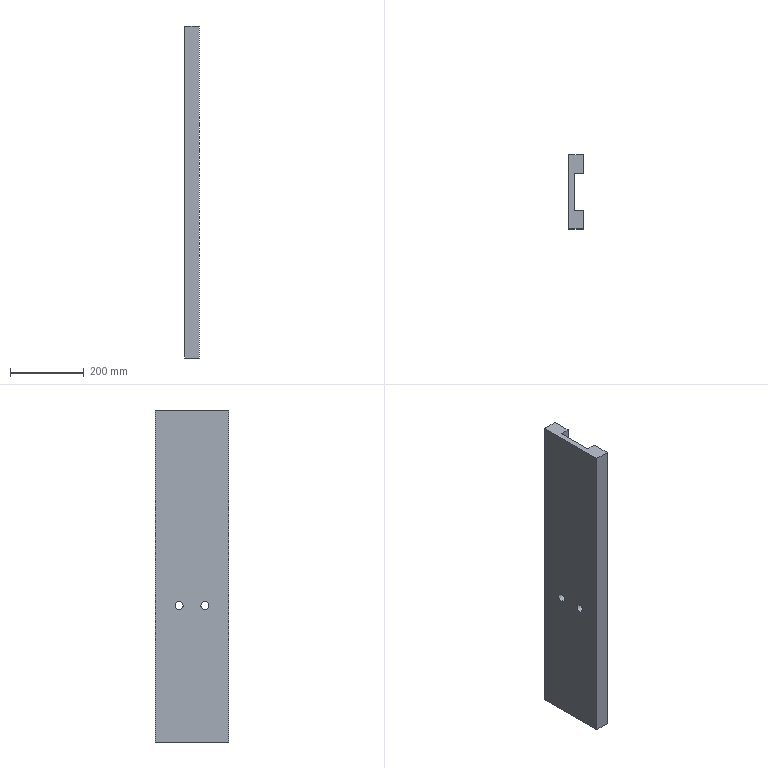Part | SolidWorks | features 3DProfileFeature 1, Extrusion 1, HoleWzd 1 | 1 solid | 14 faces | box 40 x 200 x 900 mm | volume 4927112 mm3 | plane 10 | cylinder 4 | commonest cylinder face diameters 22.225 x4
STEP:
#1=CARTESIAN_POINT('',(0.,135.,381.112));
#2=VERTEX_POINT('',#1);
#3=CARTESIAN_POINT('',(0.,135.,358.888));
#4=VERTEX_POINT('',#3);
#5=CARTESIAN_POINT('',(0.,135.,370.));
#6=DIRECTION('',(1.,0.,0.));
#7=DIRECTION('',(0.,0.,-1.));
#8=AXIS2_PLACEMENT_3D('',#5,#6,#7);
#9=CIRCLE('',#8,11.112);
#10=EDGE_CURVE('',#2,#4,#9,.T.);
#11=ORIENTED_EDGE('',*,*,#10,.F.);
#12=CARTESIAN_POINT('',(15.,135.,381.112));
#13=VERTEX_POINT('',#12);
#14=CARTESIAN_POINT('',(15.,135.,381.112));
#15=DIRECTION('',(1.,0.,0.));
#16=VECTOR('',#15,1000.);
#17=LINE('',#14,#16);
#18=EDGE_CURVE('',#2,#13,#17,.T.);
#19=ORIENTED_EDGE('',*,*,#18,.T.);
#20=CARTESIAN_POINT('',(15.,135.,358.888));
#21=VERTEX_POINT('',#20);
#22=CARTESIAN_POINT('',(15.,135.,370.));
#23=DIRECTION('',(1.,0.,0.));
#24=DIRECTION('',(0.,0.,-1.));
#25=AXIS2_PLACEMENT_3D('',#22,#23,#24);
#26=CIRCLE('',#25,11.112);
#27=EDGE_CURVE('',#13,#21,#26,.T.);
#28=ORIENTED_EDGE('',*,*,#27,.T.);
#29=CARTESIAN_POINT('',(15.,135.,358.888));
#30=DIRECTION('',(1.,0.,0.));
#31=VECTOR('',#30,1000.);
#32=LINE('',#29,#31);
#33=EDGE_CURVE('',#4,#21,#32,.T.);
#34=ORIENTED_EDGE('',*,*,#33,.F.);
#35=EDGE_LOOP('',(#11,#19,#28,#34));
#36=FACE_OUTER_BOUND('',#35,.T.);
#37=CARTESIAN_POINT('',(15.,135.,370.));
#38=DIRECTION('',(1.,0.,0.));
#39=DIRECTION('',(0.,0.,-1.));
#40=AXIS2_PLACEMENT_3D('',#37,#38,#39);
#41=CYLINDRICAL_SURFACE('',#40,11.112);
#42=ADVANCED_FACE('',(#36),#41,.F.);
#43=CARTESIAN_POINT('',(0.,65.,381.112));
#44=VERTEX_POINT('',#43);
#45=CARTESIAN_POINT('',(0.,65.,358.888));
#46=VERTEX_POINT('',#45);
#47=CARTESIAN_POINT('',(0.,65.,370.));
#48=DIRECTION('',(1.,0.,0.));
#49=DIRECTION('',(0.,0.,-1.));
#50=AXIS2_PLACEMENT_3D('',#47,#48,#49);
#51=CIRCLE('',#50,11.112);
#52=EDGE_CURVE('',#44,#46,#51,.T.);
#53=ORIENTED_EDGE('',*,*,#52,.F.);
#54=CARTESIAN_POINT('',(15.,65.,381.112));
#55=VERTEX_POINT('',#54);
#56=CARTESIAN_POINT('',(15.,65.,381.112));
#57=DIRECTION('',(1.,0.,0.));
#58=VECTOR('',#57,1000.);
#59=LINE('',#56,#58);
#60=EDGE_CURVE('',#44,#55,#59,.T.);
#61=ORIENTED_EDGE('',*,*,#60,.T.);
#62=CARTESIAN_POINT('',(15.,65.,358.888));
#63=VERTEX_POINT('',#62);
#64=CARTESIAN_POINT('',(15.,65.,370.));
#65=DIRECTION('',(1.,0.,0.));
#66=DIRECTION('',(0.,0.,-1.));
#67=AXIS2_PLACEMENT_3D('',#64,#65,#66);
#68=CIRCLE('',#67,11.112);
#69=EDGE_CURVE('',#55,#63,#68,.T.);
#70=ORIENTED_EDGE('',*,*,#69,.T.);
#71=CARTESIAN_POINT('',(15.,65.,358.888));
#72=DIRECTION('',(1.,0.,0.));
#73=VECTOR('',#72,1000.);
#74=LINE('',#71,#73);
#75=EDGE_CURVE('',#46,#63,#74,.T.);
#76=ORIENTED_EDGE('',*,*,#75,.F.);
#77=EDGE_LOOP('',(#53,#61,#70,#76));
#78=FACE_OUTER_BOUND('',#77,.T.);
#79=CARTESIAN_POINT('',(15.,65.,370.));
#80=DIRECTION('',(1.,0.,0.));
#81=DIRECTION('',(0.,0.,-1.));
#82=AXIS2_PLACEMENT_3D('',#79,#80,#81);
#83=CYLINDRICAL_SURFACE('',#82,11.112);
#84=ADVANCED_FACE('',(#78),#83,.F.);
#85=CARTESIAN_POINT('',(0.,0.,0.));
#86=VERTEX_POINT('',#85);
#87=CARTESIAN_POINT('',(40.,0.,0.));
#88=VERTEX_POINT('',#87);
#89=CARTESIAN_POINT('',(40.,0.,0.));
#90=DIRECTION('',(1.,0.,0.));
#91=VECTOR('',#90,1000.);
#92=LINE('',#89,#91);
#93=EDGE_CURVE('',#86,#88,#92,.T.);
#94=ORIENTED_EDGE('',*,*,#93,.T.);
#95=CARTESIAN_POINT('',(40.,0.,900.));
#96=VERTEX_POINT('',#95);
#97=CARTESIAN_POINT('',(40.,0.,900.));
#98=DIRECTION('',(0.,0.,-1.));
#99=VECTOR('',#98,1000.);
#100=LINE('',#97,#99);
#101=EDGE_CURVE('',#96,#88,#100,.T.);
#102=ORIENTED_EDGE('',*,*,#101,.F.);
#103=CARTESIAN_POINT('',(0.,0.,900.));
#104=VERTEX_POINT('',#103);
#105=CARTESIAN_POINT('',(40.,0.,900.));
#106=DIRECTION('',(1.,0.,0.));
#107=VECTOR('',#106,1000.);
#108=LINE('',#105,#107);
#109=EDGE_CURVE('',#104,#96,#108,.T.);
#110=ORIENTED_EDGE('',*,*,#109,.F.);
#111=CARTESIAN_POINT('',(0.,0.,900.));
#112=DIRECTION('',(0.,0.,-1.));
#113=VECTOR('',#112,1000.);
#114=LINE('',#111,#113);
#115=EDGE_CURVE('',#104,#86,#114,.T.);
#116=ORIENTED_EDGE('',*,*,#115,.T.);
#117=EDGE_LOOP('',(#94,#102,#110,#116));
#118=FACE_OUTER_BOUND('',#117,.T.);
#119=CARTESIAN_POINT('',(40.,0.,900.));
#120=DIRECTION('',(0.,1.,0.));
#121=DIRECTION('',(-1.,0.,0.));
#122=AXIS2_PLACEMENT_3D('',#119,#120,#121);
#123=PLANE('',#122);
#124=ADVANCED_FACE('',(#118),#123,.F.);
#125=CARTESIAN_POINT('',(40.,49.75,0.));
#126=VERTEX_POINT('',#125);
#127=CARTESIAN_POINT('',(40.,49.75,0.));
#128=DIRECTION('',(0.,1.,0.));
#129=VECTOR('',#128,1000.);
#130=LINE('',#127,#129);
#131=EDGE_CURVE('',#88,#126,#130,.T.);
#132=ORIENTED_EDGE('',*,*,#131,.T.);
#133=CARTESIAN_POINT('',(40.,49.75,900.));
#134=VERTEX_POINT('',#133);
#135=CARTESIAN_POINT('',(40.,49.75,900.));
#136=DIRECTION('',(0.,0.,-1.));
#137=VECTOR('',#136,1000.);
#138=LINE('',#135,#137);
#139=EDGE_CURVE('',#134,#126,#138,.T.);
#140=ORIENTED_EDGE('',*,*,#139,.F.);
#141=CARTESIAN_POINT('',(40.,49.75,900.));
#142=DIRECTION('',(0.,1.,0.));
#143=VECTOR('',#142,1000.);
#144=LINE('',#141,#143);
#145=EDGE_CURVE('',#96,#134,#144,.T.);
#146=ORIENTED_EDGE('',*,*,#145,.F.);
#147=ORIENTED_EDGE('',*,*,#101,.T.);
#148=EDGE_LOOP('',(#132,#140,#146,#147));
#149=FACE_OUTER_BOUND('',#148,.T.);
#150=CARTESIAN_POINT('',(40.,49.75,900.));
#151=DIRECTION('',(-1.,0.,0.));
#152=DIRECTION('',(0.,-1.,0.));
#153=AXIS2_PLACEMENT_3D('',#150,#151,#152);
#154=PLANE('',#153);
#155=ADVANCED_FACE('',(#149),#154,.F.);
#156=CARTESIAN_POINT('',(15.,49.75,0.));
#157=VERTEX_POINT('',#156);
#158=CARTESIAN_POINT('',(15.,49.75,0.));
#159=DIRECTION('',(-1.,0.,0.));
#160=VECTOR('',#159,1000.);
#161=LINE('',#158,#160);
#162=EDGE_CURVE('',#126,#157,#161,.T.);
#163=ORIENTED_EDGE('',*,*,#162,.T.);
#164=CARTESIAN_POINT('',(15.,49.75,900.));
#165=VERTEX_POINT('',#164);
#166=CARTESIAN_POINT('',(15.,49.75,900.));
#167=DIRECTION('',(0.,0.,-1.));
#168=VECTOR('',#167,1000.);
#169=LINE('',#166,#168);
#170=EDGE_CURVE('',#165,#157,#169,.T.);
#171=ORIENTED_EDGE('',*,*,#170,.F.);
#172=CARTESIAN_POINT('',(15.,49.75,900.));
#173=DIRECTION('',(-1.,0.,0.));
#174=VECTOR('',#173,1000.);
#175=LINE('',#172,#174);
#176=EDGE_CURVE('',#134,#165,#175,.T.);
#177=ORIENTED_EDGE('',*,*,#176,.F.);
#178=ORIENTED_EDGE('',*,*,#139,.T.);
#179=EDGE_LOOP('',(#163,#171,#177,#178));
#180=FACE_OUTER_BOUND('',#179,.T.);
#181=CARTESIAN_POINT('',(15.,49.75,900.));
#182=DIRECTION('',(0.,-1.,0.));
#183=DIRECTION('',(0.,0.,-1.));
#184=AXIS2_PLACEMENT_3D('',#181,#182,#183);
#185=PLANE('',#184);
#186=ADVANCED_FACE('',(#180),#185,.F.);
#187=CARTESIAN_POINT('',(15.,135.,370.));
#188=DIRECTION('',(1.,0.,0.));
#189=DIRECTION('',(0.,0.,-1.));
#190=AXIS2_PLACEMENT_3D('',#187,#188,#189);
#191=CIRCLE('',#190,11.112);
#192=EDGE_CURVE('',#21,#13,#191,.T.);
#193=ORIENTED_EDGE('',*,*,#192,.F.);
#194=ORIENTED_EDGE('',*,*,#27,.F.);
#195=EDGE_LOOP('',(#193,#194));
#196=FACE_BOUND('',#195,.T.);
#197=CARTESIAN_POINT('',(15.,65.,370.));
#198=DIRECTION('',(1.,0.,0.));
#199=DIRECTION('',(0.,0.,-1.));
#200=AXIS2_PLACEMENT_3D('',#197,#198,#199);
#201=CIRCLE('',#200,11.112);
#202=EDGE_CURVE('',#63,#55,#201,.T.);
#203=ORIENTED_EDGE('',*,*,#202,.F.);
#204=ORIENTED_EDGE('',*,*,#69,.F.);
#205=EDGE_LOOP('',(#203,#204));
#206=FACE_BOUND('',#205,.T.);
#207=CARTESIAN_POINT('',(15.,150.25,0.));
#208=VERTEX_POINT('',#207);
#209=CARTESIAN_POINT('',(15.,150.25,0.));
#210=DIRECTION('',(0.,1.,0.));
#211=VECTOR('',#210,1000.);
#212=LINE('',#209,#211);
#213=EDGE_CURVE('',#157,#208,#212,.T.);
#214=ORIENTED_EDGE('',*,*,#213,.T.);
#215=CARTESIAN_POINT('',(15.,150.25,900.));
#216=VERTEX_POINT('',#215);
#217=CARTESIAN_POINT('',(15.,150.25,900.));
#218=DIRECTION('',(0.,0.,-1.));
#219=VECTOR('',#218,1000.);
#220=LINE('',#217,#219);
#221=EDGE_CURVE('',#216,#208,#220,.T.);
#222=ORIENTED_EDGE('',*,*,#221,.F.);
#223=CARTESIAN_POINT('',(15.,150.25,900.));
#224=DIRECTION('',(0.,1.,0.));
#225=VECTOR('',#224,1000.);
#226=LINE('',#223,#225);
#227=EDGE_CURVE('',#165,#216,#226,.T.);
#228=ORIENTED_EDGE('',*,*,#227,.F.);
#229=ORIENTED_EDGE('',*,*,#170,.T.);
#230=EDGE_LOOP('',(#214,#222,#228,#229));
#231=FACE_OUTER_BOUND('',#230,.T.);
#232=CARTESIAN_POINT('',(15.,150.25,900.));
#233=DIRECTION('',(-1.,0.,0.));
#234=DIRECTION('',(0.,-1.,0.));
#235=AXIS2_PLACEMENT_3D('',#232,#233,#234);
#236=PLANE('',#235);
#237=ADVANCED_FACE('',(#196,#206,#231),#236,.F.);
#238=CARTESIAN_POINT('',(40.,150.25,0.));
#239=VERTEX_POINT('',#238);
#240=CARTESIAN_POINT('',(40.,150.25,0.));
#241=DIRECTION('',(1.,0.,0.));
#242=VECTOR('',#241,1000.);
#243=LINE('',#240,#242);
#244=EDGE_CURVE('',#208,#239,#243,.T.);
#245=ORIENTED_EDGE('',*,*,#244,.T.);
#246=CARTESIAN_POINT('',(40.,150.25,900.));
#247=VERTEX_POINT('',#246);
#248=CARTESIAN_POINT('',(40.,150.25,900.));
#249=DIRECTION('',(0.,0.,-1.));
#250=VECTOR('',#249,1000.);
#251=LINE('',#248,#250);
#252=EDGE_CURVE('',#247,#239,#251,.T.);
#253=ORIENTED_EDGE('',*,*,#252,.F.);
#254=CARTESIAN_POINT('',(40.,150.25,900.));
#255=DIRECTION('',(1.,0.,0.));
#256=VECTOR('',#255,1000.);
#257=LINE('',#254,#256);
#258=EDGE_CURVE('',#216,#247,#257,.T.);
#259=ORIENTED_EDGE('',*,*,#258,.F.);
#260=ORIENTED_EDGE('',*,*,#221,.T.);
#261=EDGE_LOOP('',(#245,#253,#259,#260));
#262=FACE_OUTER_BOUND('',#261,.T.);
#263=CARTESIAN_POINT('',(40.,150.25,900.));
#264=DIRECTION('',(0.,1.,0.));
#265=DIRECTION('',(0.,0.,1.));
#266=AXIS2_PLACEMENT_3D('',#263,#264,#265);
#267=PLANE('',#266);
#268=ADVANCED_FACE('',(#262),#267,.F.);
#269=CARTESIAN_POINT('',(40.,200.,0.));
#270=VERTEX_POINT('',#269);
#271=CARTESIAN_POINT('',(40.,200.,0.));
#272=DIRECTION('',(0.,1.,0.));
#273=VECTOR('',#272,1000.);
#274=LINE('',#271,#273);
#275=EDGE_CURVE('',#239,#270,#274,.T.);
#276=ORIENTED_EDGE('',*,*,#275,.T.);
#277=CARTESIAN_POINT('',(40.,200.,900.));
#278=VERTEX_POINT('',#277);
#279=CARTESIAN_POINT('',(40.,200.,900.));
#280=DIRECTION('',(0.,0.,-1.));
#281=VECTOR('',#280,1000.);
#282=LINE('',#279,#281);
#283=EDGE_CURVE('',#278,#270,#282,.T.);
#284=ORIENTED_EDGE('',*,*,#283,.F.);
#285=CARTESIAN_POINT('',(40.,200.,900.));
#286=DIRECTION('',(0.,1.,0.));
#287=VECTOR('',#286,1000.);
#288=LINE('',#285,#287);
#289=EDGE_CURVE('',#247,#278,#288,.T.);
#290=ORIENTED_EDGE('',*,*,#289,.F.);
#291=ORIENTED_EDGE('',*,*,#252,.T.);
#292=EDGE_LOOP('',(#276,#284,#290,#291));
#293=FACE_OUTER_BOUND('',#292,.T.);
#294=CARTESIAN_POINT('',(40.,200.,900.));
#295=DIRECTION('',(-1.,0.,0.));
#296=DIRECTION('',(0.,-1.,0.));
#297=AXIS2_PLACEMENT_3D('',#294,#295,#296);
#298=PLANE('',#297);
#299=ADVANCED_FACE('',(#293),#298,.F.);
#300=CARTESIAN_POINT('',(0.,200.,0.));
#301=VERTEX_POINT('',#300);
#302=CARTESIAN_POINT('',(0.,200.,0.));
#303=DIRECTION('',(-1.,0.,0.));
#304=VECTOR('',#303,1000.);
#305=LINE('',#302,#304);
#306=EDGE_CURVE('',#270,#301,#305,.T.);
#307=ORIENTED_EDGE('',*,*,#306,.T.);
#308=CARTESIAN_POINT('',(0.,200.,900.));
#309=VERTEX_POINT('',#308);
#310=CARTESIAN_POINT('',(0.,200.,900.));
#311=DIRECTION('',(0.,0.,-1.));
#312=VECTOR('',#311,1000.);
#313=LINE('',#310,#312);
#314=EDGE_CURVE('',#309,#301,#313,.T.);
#315=ORIENTED_EDGE('',*,*,#314,.F.);
#316=CARTESIAN_POINT('',(0.,200.,900.));
#317=DIRECTION('',(-1.,0.,0.));
#318=VECTOR('',#317,1000.);
#319=LINE('',#316,#318);
#320=EDGE_CURVE('',#278,#309,#319,.T.);
#321=ORIENTED_EDGE('',*,*,#320,.F.);
#322=ORIENTED_EDGE('',*,*,#283,.T.);
#323=EDGE_LOOP('',(#307,#315,#321,#322));
#324=FACE_OUTER_BOUND('',#323,.T.);
#325=CARTESIAN_POINT('',(0.,200.,900.));
#326=DIRECTION('',(0.,-1.,0.));
#327=DIRECTION('',(0.,0.,-1.));
#328=AXIS2_PLACEMENT_3D('',#325,#326,#327);
#329=PLANE('',#328);
#330=ADVANCED_FACE('',(#324),#329,.F.);
#331=CARTESIAN_POINT('',(0.,135.,370.));
#332=DIRECTION('',(1.,0.,0.));
#333=DIRECTION('',(0.,0.,-1.));
#334=AXIS2_PLACEMENT_3D('',#331,#332,#333);
#335=CIRCLE('',#334,11.112);
#336=EDGE_CURVE('',#4,#2,#335,.T.);
#337=ORIENTED_EDGE('',*,*,#336,.T.);
#338=ORIENTED_EDGE('',*,*,#10,.T.);
#339=EDGE_LOOP('',(#337,#338));
#340=FACE_BOUND('',#339,.T.);
#341=CARTESIAN_POINT('',(0.,65.,370.));
#342=DIRECTION('',(1.,0.,0.));
#343=DIRECTION('',(0.,0.,-1.));
#344=AXIS2_PLACEMENT_3D('',#341,#342,#343);
#345=CIRCLE('',#344,11.112);
#346=EDGE_CURVE('',#46,#44,#345,.T.);
#347=ORIENTED_EDGE('',*,*,#346,.T.);
#348=ORIENTED_EDGE('',*,*,#52,.T.);
#349=EDGE_LOOP('',(#347,#348));
#350=FACE_BOUND('',#349,.T.);
#351=CARTESIAN_POINT('',(0.,0.,0.));
#352=DIRECTION('',(0.,-1.,0.));
#353=VECTOR('',#352,1000.);
#354=LINE('',#351,#353);
#355=EDGE_CURVE('',#301,#86,#354,.T.);
#356=ORIENTED_EDGE('',*,*,#355,.T.);
#357=ORIENTED_EDGE('',*,*,#115,.F.);
#358=CARTESIAN_POINT('',(0.,0.,900.));
#359=DIRECTION('',(0.,-1.,0.));
#360=VECTOR('',#359,1000.);
#361=LINE('',#358,#360);
#362=EDGE_CURVE('',#309,#104,#361,.T.);
#363=ORIENTED_EDGE('',*,*,#362,.F.);
#364=ORIENTED_EDGE('',*,*,#314,.T.);
#365=EDGE_LOOP('',(#356,#357,#363,#364));
#366=FACE_OUTER_BOUND('',#365,.T.);
#367=CARTESIAN_POINT('',(0.,0.,900.));
#368=DIRECTION('',(1.,0.,0.));
#369=DIRECTION('',(0.,0.,-1.));
#370=AXIS2_PLACEMENT_3D('',#367,#368,#369);
#371=PLANE('',#370);
#372=ADVANCED_FACE('',(#340,#350,#366),#371,.F.);
#373=ORIENTED_EDGE('',*,*,#109,.T.);
#374=ORIENTED_EDGE('',*,*,#145,.T.);
#375=ORIENTED_EDGE('',*,*,#176,.T.);
#376=ORIENTED_EDGE('',*,*,#227,.T.);
#377=ORIENTED_EDGE('',*,*,#258,.T.);
#378=ORIENTED_EDGE('',*,*,#289,.T.);
#379=ORIENTED_EDGE('',*,*,#320,.T.);
#380=ORIENTED_EDGE('',*,*,#362,.T.);
#381=EDGE_LOOP('',(#373,#374,#375,#376,#377,#378,#379,#380));
#382=FACE_OUTER_BOUND('',#381,.T.);
#383=CARTESIAN_POINT('',(0.,0.,900.));
#384=DIRECTION('',(0.,0.,-1.));
#385=DIRECTION('',(-1.,0.,0.));
#386=AXIS2_PLACEMENT_3D('',#383,#384,#385);
#387=PLANE('',#386);
#388=ADVANCED_FACE('',(#382),#387,.F.);
#389=ORIENTED_EDGE('',*,*,#93,.F.);
#390=ORIENTED_EDGE('',*,*,#355,.F.);
#391=ORIENTED_EDGE('',*,*,#306,.F.);
#392=ORIENTED_EDGE('',*,*,#275,.F.);
#393=ORIENTED_EDGE('',*,*,#244,.F.);
#394=ORIENTED_EDGE('',*,*,#213,.F.);
#395=ORIENTED_EDGE('',*,*,#162,.F.);
#396=ORIENTED_EDGE('',*,*,#131,.F.);
#397=EDGE_LOOP('',(#389,#390,#391,#392,#393,#394,#395,#396));
#398=FACE_OUTER_BOUND('',#397,.T.);
#399=CARTESIAN_POINT('',(0.,0.,0.));
#400=DIRECTION('',(0.,0.,-1.));
#401=DIRECTION('',(-1.,0.,0.));
#402=AXIS2_PLACEMENT_3D('',#399,#400,#401);
#403=PLANE('',#402);
#404=ADVANCED_FACE('',(#398),#403,.T.);
#405=ORIENTED_EDGE('',*,*,#60,.F.);
#406=ORIENTED_EDGE('',*,*,#346,.F.);
#407=ORIENTED_EDGE('',*,*,#75,.T.);
#408=ORIENTED_EDGE('',*,*,#202,.T.);
#409=EDGE_LOOP('',(#405,#406,#407,#408));
#410=FACE_OUTER_BOUND('',#409,.T.);
#411=CARTESIAN_POINT('',(15.,65.,370.));
#412=DIRECTION('',(1.,0.,0.));
#413=DIRECTION('',(0.,0.,-1.));
#414=AXIS2_PLACEMENT_3D('',#411,#412,#413);
#415=CYLINDRICAL_SURFACE('',#414,11.112);
#416=ADVANCED_FACE('',(#410),#415,.F.);
#417=ORIENTED_EDGE('',*,*,#18,.F.);
#418=ORIENTED_EDGE('',*,*,#336,.F.);
#419=ORIENTED_EDGE('',*,*,#33,.T.);
#420=ORIENTED_EDGE('',*,*,#192,.T.);
#421=EDGE_LOOP('',(#417,#418,#419,#420));
#422=FACE_OUTER_BOUND('',#421,.T.);
#423=CARTESIAN_POINT('',(15.,135.,370.));
#424=DIRECTION('',(1.,0.,0.));
#425=DIRECTION('',(0.,0.,-1.));
#426=AXIS2_PLACEMENT_3D('',#423,#424,#425);
#427=CYLINDRICAL_SURFACE('',#426,11.112);
#428=ADVANCED_FACE('',(#422),#427,.F.);
#429=CLOSED_SHELL('',(#42,#84,#124,#155,#186,#237,#268,#299,#330,#372,#388,#404,#416,#428));
#430=MANIFOLD_SOLID_BREP('',#429);
#431=CARTESIAN_POINT('',(0.,0.,0.));
#432=DIRECTION('',(0.,0.,1.));
#433=DIRECTION('',(1.,0.,0.));
#434=AXIS2_PLACEMENT_3D('',#431,#432,#433);
#435=(LENGTH_UNIT()NAMED_UNIT(*)SI_UNIT(.MILLI.,.METRE.));
#436=UNCERTAINTY_MEASURE_WITH_UNIT(LENGTH_MEASURE(0.00001),#435,'','');
#437=(NAMED_UNIT(*)PLANE_ANGLE_UNIT()SI_UNIT($,.RADIAN.));
#438=(NAMED_UNIT(*)SI_UNIT($,.STERADIAN.)SOLID_ANGLE_UNIT());
#439=(GEOMETRIC_REPRESENTATION_CONTEXT(3)GLOBAL_UNCERTAINTY_ASSIGNED_CONTEXT((#436))GLOBAL_UNIT_ASSIGNED_CONTEXT((#435,#437,#438))REPRESENTATION_CONTEXT('',''));
#440=ADVANCED_BREP_SHAPE_REPRESENTATION('',(#430,#434),#439);